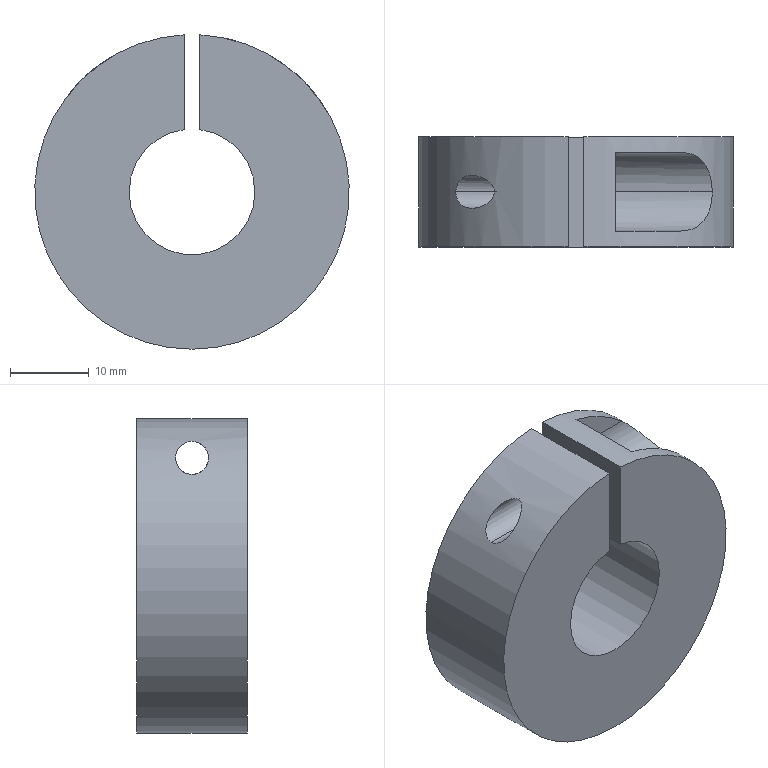Part | STEP file | A14-015 | 1 solid | 18 faces | box 40 x 14 x 39.975 mm | volume 13564 mm3 | cylinder 11 | plane 7 | commonest cylinder face diameters 2 x2 4.2 x2 5.5 x2 10 x2 40 x2 16 x1